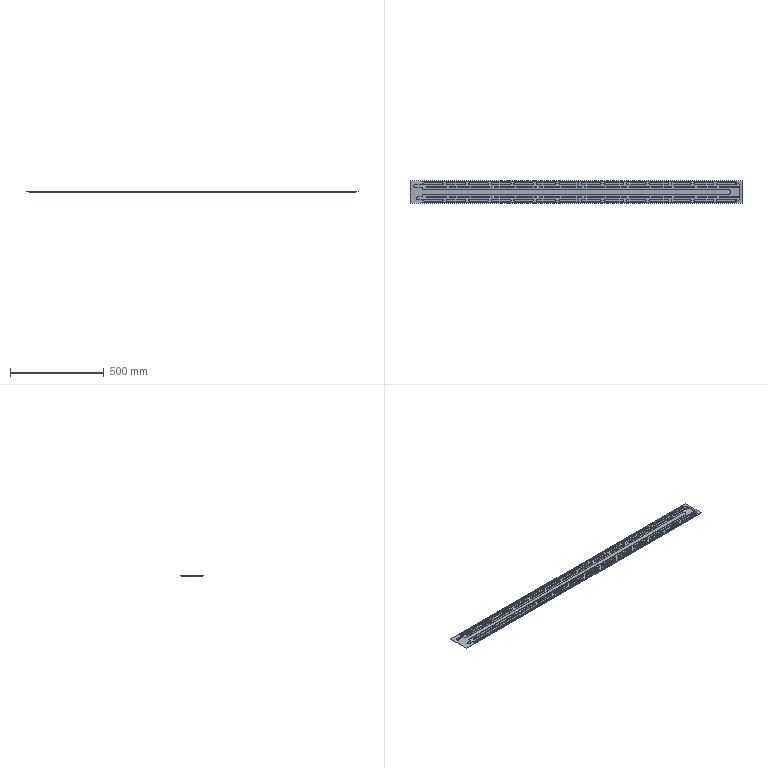Part | SolidWorks | features ICE 4, BaseBody 1, LPattern 1 | 1 solid | 716 faces | box 1768 x 120 x 5 mm | volume 357777 mm3 | plane 372 | cylinder 344 | commonest cylinder face diameters 4 x166 6 x166 12 x2 14 x2 18 x2 20 x2